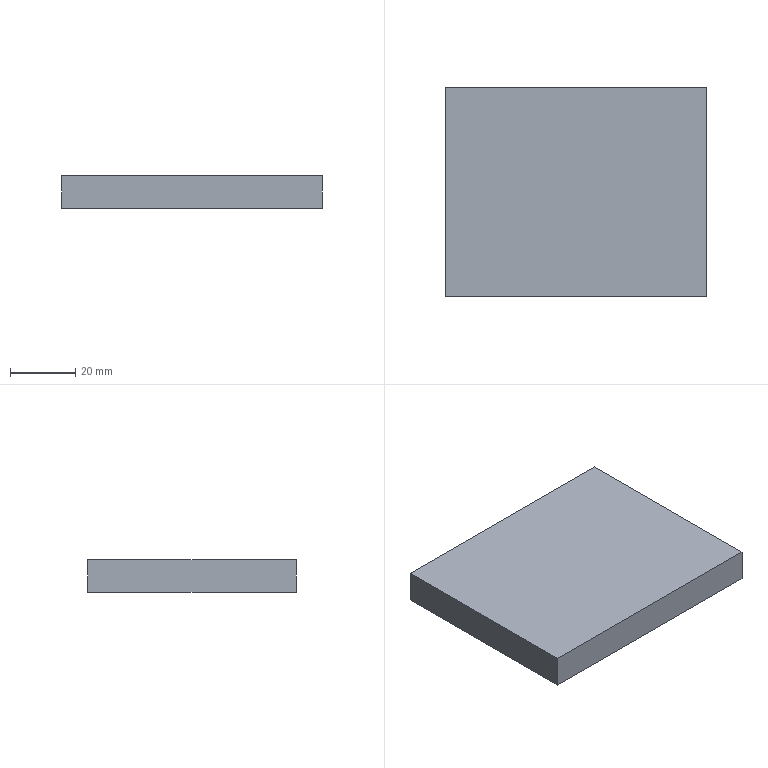Part | STEP file | Positioning_id2306_x_t | 1 solid | 6 faces | box 80 x 64 x 10 mm | volume 51200 mm3 | plane 6
STEP:
#1=CARTESIAN_POINT('',(0.,0.,0.));
#2=DIRECTION('',(0.,0.,1.));
#3=DIRECTION('',(1.,0.,0.));
#4=AXIS2_PLACEMENT_3D('',#1,#2,#3);
#5=CARTESIAN_POINT('',(-1003.002,268.,188.532));
#6=VERTEX_POINT('',#5);
#7=CARTESIAN_POINT('',(-1003.002,268.,198.532));
#8=VERTEX_POINT('',#7);
#9=CARTESIAN_POINT('',(-1003.002,268.,188.532));
#10=DIRECTION('',(0.,0.,1.));
#11=VECTOR('',#10,1.);
#12=LINE('',#9,#11);
#13=CARTESIAN_POINT('',(-1003.002,268.,193.532));
#14=DIRECTION('',(0.,-1.,0.));
#15=DIRECTION('',(1.,0.,0.));
#16=AXIS2_PLACEMENT_3D('',#13,#14,#15);
#17=PLANE('',#16);
#18=CARTESIAN_POINT('',(0.,-5.));
#19=DIRECTION('',(0.,1.));
#20=VECTOR('',#19,1.);
#21=LINE('',#18,#20);
#22=(GEOMETRIC_REPRESENTATION_CONTEXT(2)PARAMETRIC_REPRESENTATION_CONTEXT()REPRESENTATION_CONTEXT('',''));
#23=DEFINITIONAL_REPRESENTATION('',(#21),#22);
#24=PCURVE('',#17,#23);
#25=CARTESIAN_POINT('',(-1003.002,300.,193.532));
#26=DIRECTION('',(-1.,0.,0.));
#27=DIRECTION('',(0.,-1.,0.));
#28=AXIS2_PLACEMENT_3D('',#25,#26,#27);
#29=PLANE('',#28);
#30=CARTESIAN_POINT('',(32.,-5.));
#31=DIRECTION('',(0.,1.));
#32=VECTOR('',#31,1.);
#33=LINE('',#30,#32);
#34=(GEOMETRIC_REPRESENTATION_CONTEXT(2)PARAMETRIC_REPRESENTATION_CONTEXT()REPRESENTATION_CONTEXT('',''));
#35=DEFINITIONAL_REPRESENTATION('',(#33),#34);
#36=PCURVE('',#29,#35);
#37=SURFACE_CURVE('',#12,(#24,#36),.PCURVE_S1.);
#38=EDGE_CURVE('',#6,#8,#37,.T.);
#39=ORIENTED_EDGE('',*,*,#38,.F.);
#40=CARTESIAN_POINT('',(-923.002,268.,188.532));
#41=VERTEX_POINT('',#40);
#42=CARTESIAN_POINT('',(-1003.002,268.,188.532));
#43=DIRECTION('',(1.,0.,0.));
#44=VECTOR('',#43,1.);
#45=LINE('',#42,#44);
#46=CARTESIAN_POINT('',(0.,-5.));
#47=DIRECTION('',(1.,0.));
#48=VECTOR('',#47,1.);
#49=LINE('',#46,#48);
#50=(GEOMETRIC_REPRESENTATION_CONTEXT(2)PARAMETRIC_REPRESENTATION_CONTEXT()REPRESENTATION_CONTEXT('',''));
#51=DEFINITIONAL_REPRESENTATION('',(#49),#50);
#52=PCURVE('',#17,#51);
#53=CARTESIAN_POINT('',(-1003.002,300.,188.532));
#54=DIRECTION('',(0.,0.,-1.));
#55=DIRECTION('',(1.,0.,0.));
#56=AXIS2_PLACEMENT_3D('',#53,#54,#55);
#57=PLANE('',#56);
#58=CARTESIAN_POINT('',(0.,32.));
#59=DIRECTION('',(1.,0.));
#60=VECTOR('',#59,1.);
#61=LINE('',#58,#60);
#62=(GEOMETRIC_REPRESENTATION_CONTEXT(2)PARAMETRIC_REPRESENTATION_CONTEXT()REPRESENTATION_CONTEXT('',''));
#63=DEFINITIONAL_REPRESENTATION('',(#61),#62);
#64=PCURVE('',#57,#63);
#65=SURFACE_CURVE('',#45,(#52,#64),.PCURVE_S1.);
#66=EDGE_CURVE('',#6,#41,#65,.T.);
#67=ORIENTED_EDGE('',*,*,#66,.T.);
#68=CARTESIAN_POINT('',(-923.002,268.,198.532));
#69=VERTEX_POINT('',#68);
#70=CARTESIAN_POINT('',(-923.002,268.,198.532));
#71=DIRECTION('',(0.,0.,-1.));
#72=VECTOR('',#71,1.);
#73=LINE('',#70,#72);
#74=CARTESIAN_POINT('',(80.,5.));
#75=DIRECTION('',(0.,-1.));
#76=VECTOR('',#75,1.);
#77=LINE('',#74,#76);
#78=(GEOMETRIC_REPRESENTATION_CONTEXT(2)PARAMETRIC_REPRESENTATION_CONTEXT()REPRESENTATION_CONTEXT('',''));
#79=DEFINITIONAL_REPRESENTATION('',(#77),#78);
#80=PCURVE('',#17,#79);
#81=CARTESIAN_POINT('',(-923.002,300.,193.532));
#82=DIRECTION('',(1.,0.,0.));
#83=DIRECTION('',(0.,1.,0.));
#84=AXIS2_PLACEMENT_3D('',#81,#82,#83);
#85=PLANE('',#84);
#86=CARTESIAN_POINT('',(-32.,5.));
#87=DIRECTION('',(0.,-1.));
#88=VECTOR('',#87,1.);
#89=LINE('',#86,#88);
#90=(GEOMETRIC_REPRESENTATION_CONTEXT(2)PARAMETRIC_REPRESENTATION_CONTEXT()REPRESENTATION_CONTEXT('',''));
#91=DEFINITIONAL_REPRESENTATION('',(#89),#90);
#92=PCURVE('',#85,#91);
#93=SURFACE_CURVE('',#73,(#80,#92),.PCURVE_S1.);
#94=EDGE_CURVE('',#69,#41,#93,.T.);
#95=ORIENTED_EDGE('',*,*,#94,.F.);
#96=CARTESIAN_POINT('',(-1003.002,268.,198.532));
#97=DIRECTION('',(1.,0.,0.));
#98=VECTOR('',#97,1.);
#99=LINE('',#96,#98);
#100=CARTESIAN_POINT('',(0.,5.));
#101=DIRECTION('',(1.,0.));
#102=VECTOR('',#101,1.);
#103=LINE('',#100,#102);
#104=(GEOMETRIC_REPRESENTATION_CONTEXT(2)PARAMETRIC_REPRESENTATION_CONTEXT()REPRESENTATION_CONTEXT('',''));
#105=DEFINITIONAL_REPRESENTATION('',(#103),#104);
#106=PCURVE('',#17,#105);
#107=CARTESIAN_POINT('',(-1003.002,300.,198.532));
#108=DIRECTION('',(0.,0.,1.));
#109=DIRECTION('',(-1.,0.,0.));
#110=AXIS2_PLACEMENT_3D('',#107,#108,#109);
#111=PLANE('',#110);
#112=CARTESIAN_POINT('',(0.,32.));
#113=DIRECTION('',(-1.,0.));
#114=VECTOR('',#113,1.);
#115=LINE('',#112,#114);
#116=(GEOMETRIC_REPRESENTATION_CONTEXT(2)PARAMETRIC_REPRESENTATION_CONTEXT()REPRESENTATION_CONTEXT('',''));
#117=DEFINITIONAL_REPRESENTATION('',(#115),#116);
#118=PCURVE('',#111,#117);
#119=SURFACE_CURVE('',#99,(#106,#118),.PCURVE_S1.);
#120=EDGE_CURVE('',#8,#69,#119,.T.);
#121=ORIENTED_EDGE('',*,*,#120,.F.);
#122=EDGE_LOOP('',(#39,#67,#95,#121));
#123=FACE_BOUND('',#122,.T.);
#124=ADVANCED_FACE('',(#123),#17,.T.);
#125=ORIENTED_EDGE('',*,*,#38,.T.);
#126=CARTESIAN_POINT('',(-1003.002,332.,198.532));
#127=VERTEX_POINT('',#126);
#128=CARTESIAN_POINT('',(-1003.002,268.,198.532));
#129=DIRECTION('',(0.,1.,0.));
#130=VECTOR('',#129,1.);
#131=LINE('',#128,#130);
#132=CARTESIAN_POINT('',(32.,5.));
#133=DIRECTION('',(-1.,0.));
#134=VECTOR('',#133,1.);
#135=LINE('',#132,#134);
#136=(GEOMETRIC_REPRESENTATION_CONTEXT(2)PARAMETRIC_REPRESENTATION_CONTEXT()REPRESENTATION_CONTEXT('',''));
#137=DEFINITIONAL_REPRESENTATION('',(#135),#136);
#138=PCURVE('',#29,#137);
#139=CARTESIAN_POINT('',(0.,32.));
#140=DIRECTION('',(0.,-1.));
#141=VECTOR('',#140,1.);
#142=LINE('',#139,#141);
#143=(GEOMETRIC_REPRESENTATION_CONTEXT(2)PARAMETRIC_REPRESENTATION_CONTEXT()REPRESENTATION_CONTEXT('',''));
#144=DEFINITIONAL_REPRESENTATION('',(#142),#143);
#145=PCURVE('',#111,#144);
#146=SURFACE_CURVE('',#131,(#138,#145),.PCURVE_S1.);
#147=EDGE_CURVE('',#8,#127,#146,.T.);
#148=ORIENTED_EDGE('',*,*,#147,.T.);
#149=CARTESIAN_POINT('',(-1003.002,332.,188.532));
#150=VERTEX_POINT('',#149);
#151=CARTESIAN_POINT('',(-1003.002,332.,198.532));
#152=DIRECTION('',(0.,0.,-1.));
#153=VECTOR('',#152,1.);
#154=LINE('',#151,#153);
#155=CARTESIAN_POINT('',(-32.,5.));
#156=DIRECTION('',(0.,-1.));
#157=VECTOR('',#156,1.);
#158=LINE('',#155,#157);
#159=(GEOMETRIC_REPRESENTATION_CONTEXT(2)PARAMETRIC_REPRESENTATION_CONTEXT()REPRESENTATION_CONTEXT('',''));
#160=DEFINITIONAL_REPRESENTATION('',(#158),#159);
#161=PCURVE('',#29,#160);
#162=CARTESIAN_POINT('',(-1003.002,332.,193.532));
#163=DIRECTION('',(0.,1.,0.));
#164=DIRECTION('',(-1.,0.,0.));
#165=AXIS2_PLACEMENT_3D('',#162,#163,#164);
#166=PLANE('',#165);
#167=CARTESIAN_POINT('',(0.,5.));
#168=DIRECTION('',(0.,-1.));
#169=VECTOR('',#168,1.);
#170=LINE('',#167,#169);
#171=(GEOMETRIC_REPRESENTATION_CONTEXT(2)PARAMETRIC_REPRESENTATION_CONTEXT()REPRESENTATION_CONTEXT('',''));
#172=DEFINITIONAL_REPRESENTATION('',(#170),#171);
#173=PCURVE('',#166,#172);
#174=SURFACE_CURVE('',#154,(#161,#173),.PCURVE_S1.);
#175=EDGE_CURVE('',#127,#150,#174,.T.);
#176=ORIENTED_EDGE('',*,*,#175,.T.);
#177=CARTESIAN_POINT('',(-1003.002,332.,188.532));
#178=DIRECTION('',(0.,-1.,0.));
#179=VECTOR('',#178,1.);
#180=LINE('',#177,#179);
#181=CARTESIAN_POINT('',(-32.,-5.));
#182=DIRECTION('',(1.,0.));
#183=VECTOR('',#182,1.);
#184=LINE('',#181,#183);
#185=(GEOMETRIC_REPRESENTATION_CONTEXT(2)PARAMETRIC_REPRESENTATION_CONTEXT()REPRESENTATION_CONTEXT('',''));
#186=DEFINITIONAL_REPRESENTATION('',(#184),#185);
#187=PCURVE('',#29,#186);
#188=CARTESIAN_POINT('',(0.,-32.));
#189=DIRECTION('',(0.,1.));
#190=VECTOR('',#189,1.);
#191=LINE('',#188,#190);
#192=(GEOMETRIC_REPRESENTATION_CONTEXT(2)PARAMETRIC_REPRESENTATION_CONTEXT()REPRESENTATION_CONTEXT('',''));
#193=DEFINITIONAL_REPRESENTATION('',(#191),#192);
#194=PCURVE('',#57,#193);
#195=SURFACE_CURVE('',#180,(#187,#194),.PCURVE_S1.);
#196=EDGE_CURVE('',#150,#6,#195,.T.);
#197=ORIENTED_EDGE('',*,*,#196,.T.);
#198=EDGE_LOOP('',(#125,#148,#176,#197));
#199=FACE_BOUND('',#198,.T.);
#200=ADVANCED_FACE('',(#199),#29,.T.);
#201=CARTESIAN_POINT('',(-923.002,332.,198.532));
#202=VERTEX_POINT('',#201);
#203=CARTESIAN_POINT('',(-1003.002,332.,198.532));
#204=DIRECTION('',(1.,0.,0.));
#205=VECTOR('',#204,1.);
#206=LINE('',#203,#205);
#207=CARTESIAN_POINT('',(0.,-32.));
#208=DIRECTION('',(-1.,0.));
#209=VECTOR('',#208,1.);
#210=LINE('',#207,#209);
#211=(GEOMETRIC_REPRESENTATION_CONTEXT(2)PARAMETRIC_REPRESENTATION_CONTEXT()REPRESENTATION_CONTEXT('',''));
#212=DEFINITIONAL_REPRESENTATION('',(#210),#211);
#213=PCURVE('',#111,#212);
#214=CARTESIAN_POINT('',(0.,5.));
#215=DIRECTION('',(-1.,0.));
#216=VECTOR('',#215,1.);
#217=LINE('',#214,#216);
#218=(GEOMETRIC_REPRESENTATION_CONTEXT(2)PARAMETRIC_REPRESENTATION_CONTEXT()REPRESENTATION_CONTEXT('',''));
#219=DEFINITIONAL_REPRESENTATION('',(#217),#218);
#220=PCURVE('',#166,#219);
#221=SURFACE_CURVE('',#206,(#213,#220),.PCURVE_S1.);
#222=EDGE_CURVE('',#127,#202,#221,.T.);
#223=ORIENTED_EDGE('',*,*,#222,.F.);
#224=ORIENTED_EDGE('',*,*,#147,.F.);
#225=ORIENTED_EDGE('',*,*,#120,.T.);
#226=CARTESIAN_POINT('',(-923.002,332.,198.532));
#227=DIRECTION('',(0.,-1.,0.));
#228=VECTOR('',#227,1.);
#229=LINE('',#226,#228);
#230=CARTESIAN_POINT('',(-80.,-32.));
#231=DIRECTION('',(0.,1.));
#232=VECTOR('',#231,1.);
#233=LINE('',#230,#232);
#234=(GEOMETRIC_REPRESENTATION_CONTEXT(2)PARAMETRIC_REPRESENTATION_CONTEXT()REPRESENTATION_CONTEXT('',''));
#235=DEFINITIONAL_REPRESENTATION('',(#233),#234);
#236=PCURVE('',#111,#235);
#237=CARTESIAN_POINT('',(32.,5.));
#238=DIRECTION('',(-1.,0.));
#239=VECTOR('',#238,1.);
#240=LINE('',#237,#239);
#241=(GEOMETRIC_REPRESENTATION_CONTEXT(2)PARAMETRIC_REPRESENTATION_CONTEXT()REPRESENTATION_CONTEXT('',''));
#242=DEFINITIONAL_REPRESENTATION('',(#240),#241);
#243=PCURVE('',#85,#242);
#244=SURFACE_CURVE('',#229,(#236,#243),.PCURVE_S1.);
#245=EDGE_CURVE('',#202,#69,#244,.T.);
#246=ORIENTED_EDGE('',*,*,#245,.F.);
#247=EDGE_LOOP('',(#223,#224,#225,#246));
#248=FACE_BOUND('',#247,.T.);
#249=ADVANCED_FACE('',(#248),#111,.T.);
#250=CARTESIAN_POINT('',(-923.002,332.,188.532));
#251=VERTEX_POINT('',#250);
#252=CARTESIAN_POINT('',(-1003.002,332.,188.532));
#253=DIRECTION('',(1.,0.,0.));
#254=VECTOR('',#253,1.);
#255=LINE('',#252,#254);
#256=CARTESIAN_POINT('',(0.,-5.));
#257=DIRECTION('',(-1.,0.));
#258=VECTOR('',#257,1.);
#259=LINE('',#256,#258);
#260=(GEOMETRIC_REPRESENTATION_CONTEXT(2)PARAMETRIC_REPRESENTATION_CONTEXT()REPRESENTATION_CONTEXT('',''));
#261=DEFINITIONAL_REPRESENTATION('',(#259),#260);
#262=PCURVE('',#166,#261);
#263=CARTESIAN_POINT('',(0.,-32.));
#264=DIRECTION('',(1.,0.));
#265=VECTOR('',#264,1.);
#266=LINE('',#263,#265);
#267=(GEOMETRIC_REPRESENTATION_CONTEXT(2)PARAMETRIC_REPRESENTATION_CONTEXT()REPRESENTATION_CONTEXT('',''));
#268=DEFINITIONAL_REPRESENTATION('',(#266),#267);
#269=PCURVE('',#57,#268);
#270=SURFACE_CURVE('',#255,(#262,#269),.PCURVE_S1.);
#271=EDGE_CURVE('',#150,#251,#270,.T.);
#272=ORIENTED_EDGE('',*,*,#271,.F.);
#273=ORIENTED_EDGE('',*,*,#175,.F.);
#274=ORIENTED_EDGE('',*,*,#222,.T.);
#275=CARTESIAN_POINT('',(-923.002,332.,188.532));
#276=DIRECTION('',(0.,0.,1.));
#277=VECTOR('',#276,1.);
#278=LINE('',#275,#277);
#279=CARTESIAN_POINT('',(-80.,-5.));
#280=DIRECTION('',(0.,1.));
#281=VECTOR('',#280,1.);
#282=LINE('',#279,#281);
#283=(GEOMETRIC_REPRESENTATION_CONTEXT(2)PARAMETRIC_REPRESENTATION_CONTEXT()REPRESENTATION_CONTEXT('',''));
#284=DEFINITIONAL_REPRESENTATION('',(#282),#283);
#285=PCURVE('',#166,#284);
#286=CARTESIAN_POINT('',(32.,-5.));
#287=DIRECTION('',(0.,1.));
#288=VECTOR('',#287,1.);
#289=LINE('',#286,#288);
#290=(GEOMETRIC_REPRESENTATION_CONTEXT(2)PARAMETRIC_REPRESENTATION_CONTEXT()REPRESENTATION_CONTEXT('',''));
#291=DEFINITIONAL_REPRESENTATION('',(#289),#290);
#292=PCURVE('',#85,#291);
#293=SURFACE_CURVE('',#278,(#285,#292),.PCURVE_S1.);
#294=EDGE_CURVE('',#251,#202,#293,.T.);
#295=ORIENTED_EDGE('',*,*,#294,.F.);
#296=EDGE_LOOP('',(#272,#273,#274,#295));
#297=FACE_BOUND('',#296,.T.);
#298=ADVANCED_FACE('',(#297),#166,.T.);
#299=ORIENTED_EDGE('',*,*,#66,.F.);
#300=ORIENTED_EDGE('',*,*,#196,.F.);
#301=ORIENTED_EDGE('',*,*,#271,.T.);
#302=CARTESIAN_POINT('',(-923.002,268.,188.532));
#303=DIRECTION('',(0.,1.,0.));
#304=VECTOR('',#303,1.);
#305=LINE('',#302,#304);
#306=CARTESIAN_POINT('',(80.,32.));
#307=DIRECTION('',(0.,-1.));
#308=VECTOR('',#307,1.);
#309=LINE('',#306,#308);
#310=(GEOMETRIC_REPRESENTATION_CONTEXT(2)PARAMETRIC_REPRESENTATION_CONTEXT()REPRESENTATION_CONTEXT('',''));
#311=DEFINITIONAL_REPRESENTATION('',(#309),#310);
#312=PCURVE('',#57,#311);
#313=CARTESIAN_POINT('',(-32.,-5.));
#314=DIRECTION('',(1.,0.));
#315=VECTOR('',#314,1.);
#316=LINE('',#313,#315);
#317=(GEOMETRIC_REPRESENTATION_CONTEXT(2)PARAMETRIC_REPRESENTATION_CONTEXT()REPRESENTATION_CONTEXT('',''));
#318=DEFINITIONAL_REPRESENTATION('',(#316),#317);
#319=PCURVE('',#85,#318);
#320=SURFACE_CURVE('',#305,(#312,#319),.PCURVE_S1.);
#321=EDGE_CURVE('',#41,#251,#320,.T.);
#322=ORIENTED_EDGE('',*,*,#321,.F.);
#323=EDGE_LOOP('',(#299,#300,#301,#322));
#324=FACE_BOUND('',#323,.T.);
#325=ADVANCED_FACE('',(#324),#57,.T.);
#326=ORIENTED_EDGE('',*,*,#321,.T.);
#327=ORIENTED_EDGE('',*,*,#294,.T.);
#328=ORIENTED_EDGE('',*,*,#245,.T.);
#329=ORIENTED_EDGE('',*,*,#94,.T.);
#330=EDGE_LOOP('',(#326,#327,#328,#329));
#331=FACE_BOUND('',#330,.T.);
#332=ADVANCED_FACE('',(#331),#85,.T.);
#333=CLOSED_SHELL('',(#124,#200,#249,#298,#325,#332));
#334=MANIFOLD_SOLID_BREP('',#333);
#335=(LENGTH_UNIT()NAMED_UNIT(*)SI_UNIT(.MILLI.,.METRE.));
#336=UNCERTAINTY_MEASURE_WITH_UNIT(LENGTH_MEASURE(0.0000001),#335,'','');
#337=(NAMED_UNIT(*)PLANE_ANGLE_UNIT()SI_UNIT($,.RADIAN.));
#338=(NAMED_UNIT(*)SI_UNIT($,.STERADIAN.)SOLID_ANGLE_UNIT());
#339=(GEOMETRIC_REPRESENTATION_CONTEXT(3)GLOBAL_UNCERTAINTY_ASSIGNED_CONTEXT((#336))GLOBAL_UNIT_ASSIGNED_CONTEXT((#335,#337,#338))REPRESENTATION_CONTEXT('',''));
#340=ADVANCED_BREP_SHAPE_REPRESENTATION('',(#4,#334),#339);